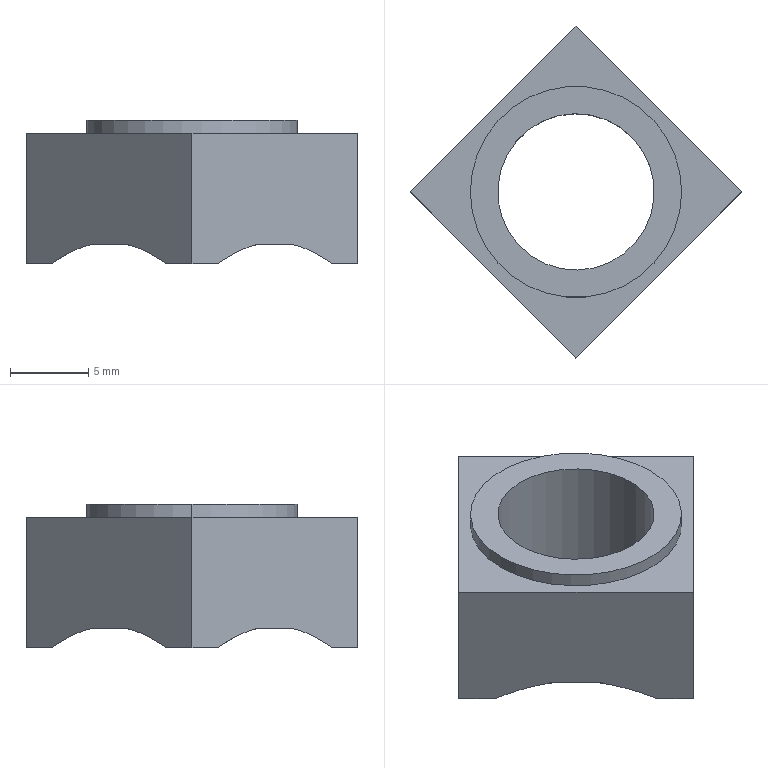Part | STEP file | Q37110 | 1 solid | 20 faces | box 21.213 x 21.213 x 9.167 mm | volume 1120 mm3 | plane 11 | cone 5 | cylinder 4 | commonest cylinder face diameters 10 x2 13.5 x2
STEP:
#1=CARTESIAN_POINT('',(4.237,6.369,0.));
#2=VERTEX_POINT('',#1);
#3=CARTESIAN_POINT('',(6.369,4.237,0.));
#4=VERTEX_POINT('',#3);
#5=CARTESIAN_POINT('',(5.303,5.303,0.));
#6=DIRECTION('',(0.7071,-0.7071,0.));
#7=VECTOR('',#6,1.);
#8=LINE('',#5,#7);
#9=EDGE_CURVE('',#2,#4,#8,.T.);
#10=ORIENTED_EDGE('',*,*,#9,.T.);
#11=CARTESIAN_POINT('',(6.714,3.668,0.));
#12=VERTEX_POINT('',#11);
#13=CARTESIAN_POINT('',(0.,0.,0.));
#14=DIRECTION('',(0.,0.,1.));
#15=AXIS2_PLACEMENT_3D('',#13,#14,$);
#16=CIRCLE('',#15,7.65);
#17=EDGE_CURVE('',#12,#4,#16,.T.);
#18=ORIENTED_EDGE('',*,*,#17,.F.);
#19=CARTESIAN_POINT('',(6.369,-4.237,0.));
#20=VERTEX_POINT('',#19);
#21=CARTESIAN_POINT('',(0.,0.,0.));
#22=DIRECTION('',(0.,0.,1.));
#23=AXIS2_PLACEMENT_3D('',#21,#22,$);
#24=CIRCLE('',#23,7.65);
#25=EDGE_CURVE('',#20,#12,#24,.T.);
#26=ORIENTED_EDGE('',*,*,#25,.F.);
#27=CARTESIAN_POINT('',(4.237,-6.369,0.));
#28=VERTEX_POINT('',#27);
#29=CARTESIAN_POINT('',(5.303,-5.303,0.));
#30=DIRECTION('',(-0.7071,-0.7071,0.));
#31=VECTOR('',#30,1.);
#32=LINE('',#29,#31);
#33=EDGE_CURVE('',#20,#28,#32,.T.);
#34=ORIENTED_EDGE('',*,*,#33,.T.);
#35=CARTESIAN_POINT('',(-4.237,-6.369,0.));
#36=VERTEX_POINT('',#35);
#37=CARTESIAN_POINT('',(0.,0.,0.));
#38=DIRECTION('',(0.,0.,1.));
#39=AXIS2_PLACEMENT_3D('',#37,#38,$);
#40=CIRCLE('',#39,7.65);
#41=EDGE_CURVE('',#36,#28,#40,.T.);
#42=ORIENTED_EDGE('',*,*,#41,.F.);
#43=CARTESIAN_POINT('',(-6.369,-4.237,0.));
#44=VERTEX_POINT('',#43);
#45=CARTESIAN_POINT('',(-5.303,-5.303,0.));
#46=DIRECTION('',(0.7071,-0.7071,0.));
#47=VECTOR('',#46,1.);
#48=LINE('',#45,#47);
#49=EDGE_CURVE('',#44,#36,#48,.T.);
#50=ORIENTED_EDGE('',*,*,#49,.F.);
#51=CARTESIAN_POINT('',(-6.714,-3.668,0.));
#52=VERTEX_POINT('',#51);
#53=CARTESIAN_POINT('',(0.,0.,0.));
#54=DIRECTION('',(0.,0.,1.));
#55=AXIS2_PLACEMENT_3D('',#53,#54,$);
#56=CIRCLE('',#55,7.65);
#57=EDGE_CURVE('',#52,#44,#56,.T.);
#58=ORIENTED_EDGE('',*,*,#57,.F.);
#59=CARTESIAN_POINT('',(-6.369,4.237,0.));
#60=VERTEX_POINT('',#59);
#61=CARTESIAN_POINT('',(0.,0.,0.));
#62=DIRECTION('',(0.,0.,1.));
#63=AXIS2_PLACEMENT_3D('',#61,#62,$);
#64=CIRCLE('',#63,7.65);
#65=EDGE_CURVE('',#60,#52,#64,.T.);
#66=ORIENTED_EDGE('',*,*,#65,.F.);
#67=CARTESIAN_POINT('',(-4.237,6.369,0.));
#68=VERTEX_POINT('',#67);
#69=CARTESIAN_POINT('',(-5.303,5.303,0.));
#70=DIRECTION('',(0.7071,0.7071,0.));
#71=VECTOR('',#70,1.);
#72=LINE('',#69,#71);
#73=EDGE_CURVE('',#60,#68,#72,.T.);
#74=ORIENTED_EDGE('',*,*,#73,.T.);
#75=CARTESIAN_POINT('',(0.,0.,0.));
#76=DIRECTION('',(0.,0.,1.));
#77=AXIS2_PLACEMENT_3D('',#75,#76,$);
#78=CIRCLE('',#77,7.65);
#79=EDGE_CURVE('',#2,#68,#78,.T.);
#80=ORIENTED_EDGE('',*,*,#79,.F.);
#81=EDGE_LOOP('',(#10,#18,#26,#34,#42,#50,#58,#66,#74,#80));
#82=FACE_OUTER_BOUND('',#81,.T.);
#83=CARTESIAN_POINT('',(-4.388,2.397,0.));
#84=VERTEX_POINT('',#83);
#85=CARTESIAN_POINT('',(4.388,-2.397,0.));
#86=VERTEX_POINT('',#85);
#87=CARTESIAN_POINT('',(0.,0.,0.));
#88=DIRECTION('',(0.,0.,1.));
#89=AXIS2_PLACEMENT_3D('',#87,#88,$);
#90=CIRCLE('',#89,5.);
#91=EDGE_CURVE('',#84,#86,#90,.T.);
#92=ORIENTED_EDGE('',*,*,#91,.T.);
#93=CARTESIAN_POINT('',(0.,0.,0.));
#94=DIRECTION('',(0.,0.,1.));
#95=AXIS2_PLACEMENT_3D('',#93,#94,$);
#96=CIRCLE('',#95,5.);
#97=EDGE_CURVE('',#86,#84,#96,.T.);
#98=ORIENTED_EDGE('',*,*,#97,.T.);
#99=EDGE_LOOP('',(#92,#98));
#100=FACE_BOUND('',#99,.T.);
#101=CARTESIAN_POINT('',(0.,0.,0.));
#102=DIRECTION('',(0.,0.,1.));
#103=DIRECTION('',(0.8333,0.,0.));
#104=AXIS2_PLACEMENT_3D('',#101,#102,#103);
#105=PLANE('',#104);
#106=ADVANCED_FACE('',(#82,#100),#105,.F.);
#107=CARTESIAN_POINT('',(-1.61,8.997,-1.25));
#108=VERTEX_POINT('',#107);
#109=CARTESIAN_POINT('',(-4.237,6.369,0.));
#110=CARTESIAN_POINT('',(-3.9,6.707,-0.07892));
#111=CARTESIAN_POINT('',(-3.552,7.054,-0.1902));
#112=CARTESIAN_POINT('',(-3.189,7.418,-0.337));
#113=CARTESIAN_POINT('',(-2.669,7.938,-0.5899));
#114=CARTESIAN_POINT('',(-2.088,8.519,-0.9383));
#115=CARTESIAN_POINT('',(-1.934,8.673,-1.035));
#116=CARTESIAN_POINT('',(-1.775,8.832,-1.138));
#117=CARTESIAN_POINT('',(-1.61,8.997,-1.25));
#118=B_SPLINE_CURVE_WITH_KNOTS('',5,(#109,#110,#111,#112,#113,#114,#115,#116,#117),.UNSPECIFIED.,.F.,.U.,(6,3,6),(0.,30.729,41.356),.UNSPECIFIED.);
#119=EDGE_CURVE('',#68,#108,#118,.T.);
#120=ORIENTED_EDGE('',*,*,#119,.F.);
#121=ORIENTED_EDGE('',*,*,#73,.F.);
#122=CARTESIAN_POINT('',(-8.997,1.61,-1.25));
#123=VERTEX_POINT('',#122);
#124=CARTESIAN_POINT('',(-6.369,4.237,0.));
#125=CARTESIAN_POINT('',(-6.707,3.9,-0.07892));
#126=CARTESIAN_POINT('',(-7.054,3.552,-0.1902));
#127=CARTESIAN_POINT('',(-7.418,3.189,-0.337));
#128=CARTESIAN_POINT('',(-7.938,2.669,-0.5899));
#129=CARTESIAN_POINT('',(-8.519,2.088,-0.9383));
#130=CARTESIAN_POINT('',(-8.673,1.934,-1.035));
#131=CARTESIAN_POINT('',(-8.832,1.775,-1.138));
#132=CARTESIAN_POINT('',(-8.997,1.61,-1.25));
#133=B_SPLINE_CURVE_WITH_KNOTS('',5,(#124,#125,#126,#127,#128,#129,#130,#131,#132),.UNSPECIFIED.,.F.,.U.,(6,3,6),(0.,30.729,41.356),.UNSPECIFIED.);
#134=EDGE_CURVE('',#60,#123,#133,.T.);
#135=ORIENTED_EDGE('',*,*,#134,.T.);
#136=CARTESIAN_POINT('',(-10.607,0.,-1.25));
#137=VERTEX_POINT('',#136);
#138=CARTESIAN_POINT('',(-9.802,0.8049,-1.25));
#139=DIRECTION('',(0.7071,0.7071,0.));
#140=VECTOR('',#139,1.);
#141=LINE('',#138,#140);
#142=EDGE_CURVE('',#123,#137,#141,.F.);
#143=ORIENTED_EDGE('',*,*,#142,.T.);
#144=CARTESIAN_POINT('',(-10.607,0.,7.083));
#145=VERTEX_POINT('',#144);
#146=CARTESIAN_POINT('',(-10.607,0.,2.917));
#147=DIRECTION('',(0.,0.,1.));
#148=VECTOR('',#147,1.);
#149=LINE('',#146,#148);
#150=EDGE_CURVE('',#137,#145,#149,.T.);
#151=ORIENTED_EDGE('',*,*,#150,.T.);
#152=CARTESIAN_POINT('',(0.,10.607,7.083));
#153=VERTEX_POINT('',#152);
#154=CARTESIAN_POINT('',(-5.303,5.303,7.083));
#155=DIRECTION('',(0.7071,0.7071,0.));
#156=VECTOR('',#155,1.);
#157=LINE('',#154,#156);
#158=EDGE_CURVE('',#153,#145,#157,.F.);
#159=ORIENTED_EDGE('',*,*,#158,.F.);
#160=CARTESIAN_POINT('',(0.,10.607,-1.25));
#161=VERTEX_POINT('',#160);
#162=CARTESIAN_POINT('',(0.,10.607,2.917));
#163=DIRECTION('',(0.,0.,1.));
#164=VECTOR('',#163,1.);
#165=LINE('',#162,#164);
#166=EDGE_CURVE('',#161,#153,#165,.T.);
#167=ORIENTED_EDGE('',*,*,#166,.F.);
#168=CARTESIAN_POINT('',(-0.8049,9.802,-1.25));
#169=DIRECTION('',(0.7071,0.7071,0.));
#170=VECTOR('',#169,1.);
#171=LINE('',#168,#170);
#172=EDGE_CURVE('',#161,#108,#171,.F.);
#173=ORIENTED_EDGE('',*,*,#172,.T.);
#174=EDGE_LOOP('',(#120,#121,#135,#143,#151,#159,#167,#173));
#175=FACE_OUTER_BOUND('',#174,.T.);
#176=CARTESIAN_POINT('',(-10.607,0.,0.));
#177=DIRECTION('',(0.7071,-0.7071,0.));
#178=DIRECTION('',(0.5893,0.5893,0.));
#179=AXIS2_PLACEMENT_3D('',#176,#177,#178);
#180=PLANE('',#179);
#181=ADVANCED_FACE('',(#175),#180,.F.);
#182=CARTESIAN_POINT('',(1.61,-8.997,-1.25));
#183=VERTEX_POINT('',#182);
#184=CARTESIAN_POINT('',(4.237,-6.369,0.));
#185=CARTESIAN_POINT('',(3.9,-6.707,-0.07892));
#186=CARTESIAN_POINT('',(3.552,-7.054,-0.1902));
#187=CARTESIAN_POINT('',(3.189,-7.418,-0.337));
#188=CARTESIAN_POINT('',(2.669,-7.938,-0.5899));
#189=CARTESIAN_POINT('',(2.088,-8.519,-0.9383));
#190=CARTESIAN_POINT('',(1.934,-8.673,-1.035));
#191=CARTESIAN_POINT('',(1.775,-8.832,-1.138));
#192=CARTESIAN_POINT('',(1.61,-8.997,-1.25));
#193=B_SPLINE_CURVE_WITH_KNOTS('',5,(#184,#185,#186,#187,#188,#189,#190,#191,#192),.UNSPECIFIED.,.F.,.U.,(6,3,6),(0.,30.729,41.356),.UNSPECIFIED.);
#194=EDGE_CURVE('',#28,#183,#193,.T.);
#195=ORIENTED_EDGE('',*,*,#194,.F.);
#196=ORIENTED_EDGE('',*,*,#33,.F.);
#197=CARTESIAN_POINT('',(8.997,-1.61,-1.25));
#198=VERTEX_POINT('',#197);
#199=CARTESIAN_POINT('',(6.369,-4.237,0.));
#200=CARTESIAN_POINT('',(6.707,-3.9,-0.07892));
#201=CARTESIAN_POINT('',(7.054,-3.552,-0.1902));
#202=CARTESIAN_POINT('',(7.418,-3.189,-0.337));
#203=CARTESIAN_POINT('',(7.938,-2.669,-0.5899));
#204=CARTESIAN_POINT('',(8.519,-2.088,-0.9383));
#205=CARTESIAN_POINT('',(8.673,-1.934,-1.035));
#206=CARTESIAN_POINT('',(8.832,-1.775,-1.138));
#207=CARTESIAN_POINT('',(8.997,-1.61,-1.25));
#208=B_SPLINE_CURVE_WITH_KNOTS('',5,(#199,#200,#201,#202,#203,#204,#205,#206,#207),.UNSPECIFIED.,.F.,.U.,(6,3,6),(0.,30.729,41.356),.UNSPECIFIED.);
#209=EDGE_CURVE('',#20,#198,#208,.T.);
#210=ORIENTED_EDGE('',*,*,#209,.T.);
#211=CARTESIAN_POINT('',(10.607,0.,-1.25));
#212=VERTEX_POINT('',#211);
#213=CARTESIAN_POINT('',(9.802,-0.8049,-1.25));
#214=DIRECTION('',(-0.7071,-0.7071,0.));
#215=VECTOR('',#214,1.);
#216=LINE('',#213,#215);
#217=EDGE_CURVE('',#198,#212,#216,.F.);
#218=ORIENTED_EDGE('',*,*,#217,.T.);
#219=CARTESIAN_POINT('',(10.607,0.,7.083));
#220=VERTEX_POINT('',#219);
#221=CARTESIAN_POINT('',(10.607,0.,2.917));
#222=DIRECTION('',(0.,0.,1.));
#223=VECTOR('',#222,1.);
#224=LINE('',#221,#223);
#225=EDGE_CURVE('',#212,#220,#224,.T.);
#226=ORIENTED_EDGE('',*,*,#225,.T.);
#227=CARTESIAN_POINT('',(0.,-10.607,7.083));
#228=VERTEX_POINT('',#227);
#229=CARTESIAN_POINT('',(5.303,-5.303,7.083));
#230=DIRECTION('',(-0.7071,-0.7071,0.));
#231=VECTOR('',#230,1.);
#232=LINE('',#229,#231);
#233=EDGE_CURVE('',#228,#220,#232,.F.);
#234=ORIENTED_EDGE('',*,*,#233,.F.);
#235=CARTESIAN_POINT('',(0.,-10.607,-1.25));
#236=VERTEX_POINT('',#235);
#237=CARTESIAN_POINT('',(0.,-10.607,2.917));
#238=DIRECTION('',(0.,0.,1.));
#239=VECTOR('',#238,1.);
#240=LINE('',#237,#239);
#241=EDGE_CURVE('',#236,#228,#240,.T.);
#242=ORIENTED_EDGE('',*,*,#241,.F.);
#243=CARTESIAN_POINT('',(0.8049,-9.802,-1.25));
#244=DIRECTION('',(-0.7071,-0.7071,0.));
#245=VECTOR('',#244,1.);
#246=LINE('',#243,#245);
#247=EDGE_CURVE('',#236,#183,#246,.F.);
#248=ORIENTED_EDGE('',*,*,#247,.T.);
#249=EDGE_LOOP('',(#195,#196,#210,#218,#226,#234,#242,#248));
#250=FACE_OUTER_BOUND('',#249,.T.);
#251=CARTESIAN_POINT('',(10.607,0.,0.));
#252=DIRECTION('',(-0.7071,0.7071,0.));
#253=DIRECTION('',(-0.5893,-0.5893,0.));
#254=AXIS2_PLACEMENT_3D('',#251,#252,#253);
#255=PLANE('',#254);
#256=ADVANCED_FACE('',(#250),#255,.F.);
#257=CARTESIAN_POINT('',(6.859,3.747,-0.1394));
#258=VERTEX_POINT('',#257);
#259=CARTESIAN_POINT('',(8.997,1.61,-1.25));
#260=VERTEX_POINT('',#259);
#261=CARTESIAN_POINT('',(6.859,3.747,-0.1394));
#262=CARTESIAN_POINT('',(7.213,3.394,-0.2575));
#263=CARTESIAN_POINT('',(7.581,3.025,-0.4115));
#264=CARTESIAN_POINT('',(7.972,2.634,-0.6064));
#265=CARTESIAN_POINT('',(8.418,2.188,-0.8643));
#266=CARTESIAN_POINT('',(8.915,1.691,-1.195));
#267=CARTESIAN_POINT('',(8.942,1.664,-1.213));
#268=CARTESIAN_POINT('',(8.969,1.637,-1.231));
#269=CARTESIAN_POINT('',(8.997,1.61,-1.25));
#270=B_SPLINE_CURVE_WITH_KNOTS('',5,(#261,#262,#263,#264,#265,#266,#267,#268,#269),.UNSPECIFIED.,.F.,.U.,(6,3,6),(0.,30.843,32.608),.UNSPECIFIED.);
#271=EDGE_CURVE('',#258,#260,#270,.T.);
#272=ORIENTED_EDGE('',*,*,#271,.F.);
#273=CARTESIAN_POINT('',(6.369,4.237,0.));
#274=CARTESIAN_POINT('',(6.465,4.141,-0.02247));
#275=CARTESIAN_POINT('',(6.562,4.044,-0.04757));
#276=CARTESIAN_POINT('',(6.66,3.946,-0.07536));
#277=CARTESIAN_POINT('',(6.759,3.847,-0.1059));
#278=CARTESIAN_POINT('',(6.859,3.747,-0.1394));
#279=B_SPLINE_CURVE_WITH_KNOTS('',5,(#273,#274,#275,#276,#277,#278),.UNSPECIFIED.,.F.,.U.,(6,6),(0.,8.749),.UNSPECIFIED.);
#280=EDGE_CURVE('',#4,#258,#279,.T.);
#281=ORIENTED_EDGE('',*,*,#280,.F.);
#282=ORIENTED_EDGE('',*,*,#9,.F.);
#283=CARTESIAN_POINT('',(1.61,8.997,-1.25));
#284=VERTEX_POINT('',#283);
#285=CARTESIAN_POINT('',(4.237,6.369,0.));
#286=CARTESIAN_POINT('',(3.9,6.707,-0.07892));
#287=CARTESIAN_POINT('',(3.552,7.054,-0.1902));
#288=CARTESIAN_POINT('',(3.189,7.418,-0.337));
#289=CARTESIAN_POINT('',(2.669,7.938,-0.5899));
#290=CARTESIAN_POINT('',(2.088,8.519,-0.9383));
#291=CARTESIAN_POINT('',(1.934,8.673,-1.035));
#292=CARTESIAN_POINT('',(1.775,8.832,-1.138));
#293=CARTESIAN_POINT('',(1.61,8.997,-1.25));
#294=B_SPLINE_CURVE_WITH_KNOTS('',5,(#285,#286,#287,#288,#289,#290,#291,#292,#293),.UNSPECIFIED.,.F.,.U.,(6,3,6),(0.,30.729,41.356),.UNSPECIFIED.);
#295=EDGE_CURVE('',#2,#284,#294,.T.);
#296=ORIENTED_EDGE('',*,*,#295,.T.);
#297=CARTESIAN_POINT('',(0.8049,9.802,-1.25));
#298=DIRECTION('',(0.7071,-0.7071,0.));
#299=VECTOR('',#298,1.);
#300=LINE('',#297,#299);
#301=EDGE_CURVE('',#284,#161,#300,.F.);
#302=ORIENTED_EDGE('',*,*,#301,.T.);
#303=ORIENTED_EDGE('',*,*,#166,.T.);
#304=CARTESIAN_POINT('',(5.303,5.303,7.083));
#305=DIRECTION('',(0.7071,-0.7071,0.));
#306=VECTOR('',#305,1.);
#307=LINE('',#304,#306);
#308=EDGE_CURVE('',#220,#153,#307,.F.);
#309=ORIENTED_EDGE('',*,*,#308,.F.);
#310=ORIENTED_EDGE('',*,*,#225,.F.);
#311=CARTESIAN_POINT('',(9.802,0.8049,-1.25));
#312=DIRECTION('',(0.7071,-0.7071,0.));
#313=VECTOR('',#312,1.);
#314=LINE('',#311,#313);
#315=EDGE_CURVE('',#212,#260,#314,.F.);
#316=ORIENTED_EDGE('',*,*,#315,.T.);
#317=EDGE_LOOP('',(#272,#281,#282,#296,#302,#303,#309,#310,#316));
#318=FACE_OUTER_BOUND('',#317,.T.);
#319=CARTESIAN_POINT('',(0.,10.607,0.));
#320=DIRECTION('',(-0.7071,-0.7071,0.));
#321=DIRECTION('',(0.5893,-0.5893,0.));
#322=AXIS2_PLACEMENT_3D('',#319,#320,#321);
#323=PLANE('',#322);
#324=ADVANCED_FACE('',(#318),#323,.F.);
#325=ORIENTED_EDGE('',*,*,#97,.F.);
#326=CARTESIAN_POINT('',(4.388,-2.397,7.917));
#327=VERTEX_POINT('',#326);
#328=CARTESIAN_POINT('',(4.388,-2.397,3.333));
#329=DIRECTION('',(0.,0.,-1.));
#330=VECTOR('',#329,1.);
#331=LINE('',#328,#330);
#332=EDGE_CURVE('',#86,#327,#331,.F.);
#333=ORIENTED_EDGE('',*,*,#332,.T.);
#334=CARTESIAN_POINT('',(-4.388,2.397,7.917));
#335=VERTEX_POINT('',#334);
#336=CARTESIAN_POINT('',(0.,0.,7.917));
#337=DIRECTION('',(0.,0.,-1.));
#338=AXIS2_PLACEMENT_3D('',#336,#337,$);
#339=CIRCLE('',#338,5.);
#340=EDGE_CURVE('',#327,#335,#339,.F.);
#341=ORIENTED_EDGE('',*,*,#340,.T.);
#342=CARTESIAN_POINT('',(-4.388,2.397,3.333));
#343=DIRECTION('',(0.,0.,-1.));
#344=VECTOR('',#343,1.);
#345=LINE('',#342,#344);
#346=EDGE_CURVE('',#84,#335,#345,.F.);
#347=ORIENTED_EDGE('',*,*,#346,.F.);
#348=EDGE_LOOP('',(#325,#333,#341,#347));
#349=FACE_OUTER_BOUND('',#348,.T.);
#350=CARTESIAN_POINT('',(0.,0.,7.667));
#351=DIRECTION('',(0.,0.,-1.));
#352=DIRECTION('',(0.8776,-0.4794,0.));
#353=AXIS2_PLACEMENT_3D('',#350,#351,#352);
#354=CYLINDRICAL_SURFACE('',#353,5.);
#355=ADVANCED_FACE('',(#349),#354,.F.);
#356=ORIENTED_EDGE('',*,*,#91,.F.);
#357=ORIENTED_EDGE('',*,*,#346,.T.);
#358=CARTESIAN_POINT('',(0.,0.,7.917));
#359=DIRECTION('',(0.,0.,-1.));
#360=AXIS2_PLACEMENT_3D('',#358,#359,$);
#361=CIRCLE('',#360,5.);
#362=EDGE_CURVE('',#335,#327,#361,.F.);
#363=ORIENTED_EDGE('',*,*,#362,.T.);
#364=ORIENTED_EDGE('',*,*,#332,.F.);
#365=EDGE_LOOP('',(#356,#357,#363,#364));
#366=FACE_OUTER_BOUND('',#365,.T.);
#367=ADVANCED_FACE('',(#366),#354,.F.);
#368=CARTESIAN_POINT('',(0.,0.,-1.25));
#369=DIRECTION('',(0.,0.,1.));
#370=AXIS2_PLACEMENT_3D('',#368,#369,$);
#371=CIRCLE('',#370,9.14);
#372=EDGE_CURVE('',#284,#108,#371,.T.);
#373=ORIENTED_EDGE('',*,*,#372,.T.);
#374=ORIENTED_EDGE('',*,*,#172,.F.);
#375=ORIENTED_EDGE('',*,*,#301,.F.);
#376=EDGE_LOOP('',(#373,#374,#375));
#377=FACE_OUTER_BOUND('',#376,.T.);
#378=CARTESIAN_POINT('',(0.,0.,-1.25));
#379=DIRECTION('',(0.,0.,1.));
#380=DIRECTION('',(0.8333,0.,0.));
#381=AXIS2_PLACEMENT_3D('',#378,#379,#380);
#382=PLANE('',#381);
#383=ADVANCED_FACE('',(#377),#382,.F.);
#384=CARTESIAN_POINT('',(-8.997,-1.61,-1.25));
#385=VERTEX_POINT('',#384);
#386=CARTESIAN_POINT('',(0.,0.,-1.25));
#387=DIRECTION('',(0.,0.,1.));
#388=AXIS2_PLACEMENT_3D('',#386,#387,$);
#389=CIRCLE('',#388,9.14);
#390=EDGE_CURVE('',#123,#385,#389,.T.);
#391=ORIENTED_EDGE('',*,*,#390,.T.);
#392=CARTESIAN_POINT('',(-9.802,-0.8049,-1.25));
#393=DIRECTION('',(-0.7071,0.7071,0.));
#394=VECTOR('',#393,1.);
#395=LINE('',#392,#394);
#396=EDGE_CURVE('',#137,#385,#395,.F.);
#397=ORIENTED_EDGE('',*,*,#396,.F.);
#398=ORIENTED_EDGE('',*,*,#142,.F.);
#399=EDGE_LOOP('',(#391,#397,#398));
#400=FACE_OUTER_BOUND('',#399,.T.);
#401=ADVANCED_FACE('',(#400),#382,.F.);
#402=CARTESIAN_POINT('',(-1.61,-8.997,-1.25));
#403=VERTEX_POINT('',#402);
#404=CARTESIAN_POINT('',(0.,0.,-1.25));
#405=DIRECTION('',(0.,0.,1.));
#406=AXIS2_PLACEMENT_3D('',#404,#405,$);
#407=CIRCLE('',#406,9.14);
#408=EDGE_CURVE('',#403,#183,#407,.T.);
#409=ORIENTED_EDGE('',*,*,#408,.T.);
#410=ORIENTED_EDGE('',*,*,#247,.F.);
#411=CARTESIAN_POINT('',(-0.8049,-9.802,-1.25));
#412=DIRECTION('',(-0.7071,0.7071,0.));
#413=VECTOR('',#412,1.);
#414=LINE('',#411,#413);
#415=EDGE_CURVE('',#403,#236,#414,.F.);
#416=ORIENTED_EDGE('',*,*,#415,.F.);
#417=EDGE_LOOP('',(#409,#410,#416));
#418=FACE_OUTER_BOUND('',#417,.T.);
#419=ADVANCED_FACE('',(#418),#382,.F.);
#420=CARTESIAN_POINT('',(0.,0.,-1.25));
#421=DIRECTION('',(0.,0.,1.));
#422=AXIS2_PLACEMENT_3D('',#420,#421,$);
#423=CIRCLE('',#422,9.14);
#424=EDGE_CURVE('',#198,#260,#423,.T.);
#425=ORIENTED_EDGE('',*,*,#424,.T.);
#426=ORIENTED_EDGE('',*,*,#315,.F.);
#427=ORIENTED_EDGE('',*,*,#217,.F.);
#428=EDGE_LOOP('',(#425,#426,#427));
#429=FACE_OUTER_BOUND('',#428,.T.);
#430=ADVANCED_FACE('',(#429),#382,.F.);
#431=CARTESIAN_POINT('',(6.75,0.,7.917));
#432=VERTEX_POINT('',#431);
#433=CARTESIAN_POINT('',(-6.75,0.,7.917));
#434=VERTEX_POINT('',#433);
#435=CARTESIAN_POINT('',(0.,0.,7.917));
#436=DIRECTION('',(0.,0.,1.));
#437=AXIS2_PLACEMENT_3D('',#435,#436,$);
#438=CIRCLE('',#437,6.75);
#439=EDGE_CURVE('',#432,#434,#438,.T.);
#440=ORIENTED_EDGE('',*,*,#439,.T.);
#441=CARTESIAN_POINT('',(0.,0.,7.917));
#442=DIRECTION('',(0.,0.,1.));
#443=AXIS2_PLACEMENT_3D('',#441,#442,$);
#444=CIRCLE('',#443,6.75);
#445=EDGE_CURVE('',#434,#432,#444,.T.);
#446=ORIENTED_EDGE('',*,*,#445,.T.);
#447=EDGE_LOOP('',(#440,#446));
#448=FACE_OUTER_BOUND('',#447,.T.);
#449=ORIENTED_EDGE('',*,*,#362,.F.);
#450=ORIENTED_EDGE('',*,*,#340,.F.);
#451=EDGE_LOOP('',(#449,#450));
#452=FACE_BOUND('',#451,.T.);
#453=CARTESIAN_POINT('',(0.,0.,7.917));
#454=DIRECTION('',(0.,0.,1.));
#455=DIRECTION('',(0.8333,0.,0.));
#456=AXIS2_PLACEMENT_3D('',#453,#454,#455);
#457=PLANE('',#456);
#458=ADVANCED_FACE('',(#448,#452),#457,.T.);
#459=CARTESIAN_POINT('',(6.75,0.,7.083));
#460=VERTEX_POINT('',#459);
#461=CARTESIAN_POINT('',(6.75,0.,7.5));
#462=DIRECTION('',(0.,0.,1.));
#463=VECTOR('',#462,1.);
#464=LINE('',#461,#463);
#465=EDGE_CURVE('',#460,#432,#464,.T.);
#466=ORIENTED_EDGE('',*,*,#465,.F.);
#467=CARTESIAN_POINT('',(-6.75,0.,7.083));
#468=VERTEX_POINT('',#467);
#469=CARTESIAN_POINT('',(0.,0.,7.083));
#470=DIRECTION('',(0.,0.,1.));
#471=AXIS2_PLACEMENT_3D('',#469,#470,$);
#472=CIRCLE('',#471,6.75);
#473=EDGE_CURVE('',#460,#468,#472,.T.);
#474=ORIENTED_EDGE('',*,*,#473,.T.);
#475=CARTESIAN_POINT('',(-6.75,0.,7.5));
#476=DIRECTION('',(0.,0.,1.));
#477=VECTOR('',#476,1.);
#478=LINE('',#475,#477);
#479=EDGE_CURVE('',#468,#434,#478,.T.);
#480=ORIENTED_EDGE('',*,*,#479,.T.);
#481=ORIENTED_EDGE('',*,*,#439,.F.);
#482=EDGE_LOOP('',(#466,#474,#480,#481));
#483=FACE_OUTER_BOUND('',#482,.T.);
#484=CARTESIAN_POINT('',(0.,0.,7.5));
#485=DIRECTION('',(0.,0.,1.));
#486=DIRECTION('',(1.,0.,0.));
#487=AXIS2_PLACEMENT_3D('',#484,#485,#486);
#488=CYLINDRICAL_SURFACE('',#487,6.75);
#489=ADVANCED_FACE('',(#483),#488,.T.);
#490=ORIENTED_EDGE('',*,*,#479,.F.);
#491=CARTESIAN_POINT('',(0.,0.,7.083));
#492=DIRECTION('',(0.,0.,1.));
#493=AXIS2_PLACEMENT_3D('',#491,#492,$);
#494=CIRCLE('',#493,6.75);
#495=EDGE_CURVE('',#468,#460,#494,.T.);
#496=ORIENTED_EDGE('',*,*,#495,.T.);
#497=ORIENTED_EDGE('',*,*,#465,.T.);
#498=ORIENTED_EDGE('',*,*,#445,.F.);
#499=EDGE_LOOP('',(#490,#496,#497,#498));
#500=FACE_OUTER_BOUND('',#499,.T.);
#501=ADVANCED_FACE('',(#500),#488,.T.);
#502=CARTESIAN_POINT('',(-5.303,-5.303,7.083));
#503=DIRECTION('',(-0.7071,0.7071,0.));
#504=VECTOR('',#503,1.);
#505=LINE('',#502,#504);
#506=EDGE_CURVE('',#145,#228,#505,.F.);
#507=ORIENTED_EDGE('',*,*,#506,.T.);
#508=ORIENTED_EDGE('',*,*,#233,.T.);
#509=ORIENTED_EDGE('',*,*,#308,.T.);
#510=ORIENTED_EDGE('',*,*,#158,.T.);
#511=EDGE_LOOP('',(#507,#508,#509,#510));
#512=FACE_OUTER_BOUND('',#511,.T.);
#513=ORIENTED_EDGE('',*,*,#473,.F.);
#514=ORIENTED_EDGE('',*,*,#495,.F.);
#515=EDGE_LOOP('',(#513,#514));
#516=FACE_BOUND('',#515,.T.);
#517=CARTESIAN_POINT('',(0.,0.,7.083));
#518=DIRECTION('',(0.,0.,1.));
#519=DIRECTION('',(0.8333,0.,0.));
#520=AXIS2_PLACEMENT_3D('',#517,#518,#519);
#521=PLANE('',#520);
#522=ADVANCED_FACE('',(#512,#516),#521,.T.);
#523=ORIENTED_EDGE('',*,*,#280,.T.);
#524=CARTESIAN_POINT('',(7.423,4.055,-0.6786));
#525=DIRECTION('',(0.6723,0.3673,-0.6428));
#526=VECTOR('',#525,1.);
#527=LINE('',#524,#526);
#528=EDGE_CURVE('',#12,#258,#527,.T.);
#529=ORIENTED_EDGE('',*,*,#528,.F.);
#530=ORIENTED_EDGE('',*,*,#17,.T.);
#531=EDGE_LOOP('',(#523,#529,#530));
#532=FACE_OUTER_BOUND('',#531,.T.);
#533=CARTESIAN_POINT('',(0.,0.,0.));
#534=DIRECTION('',(0.,0.,-1.));
#535=DIRECTION('',(0.8776,0.4794,0.));
#536=AXIS2_PLACEMENT_3D('',#533,#534,#535);
#537=CONICAL_SURFACE('',#536,7.65,0.8727);
#538=ADVANCED_FACE('',(#532),#537,.F.);
#539=ORIENTED_EDGE('',*,*,#271,.T.);
#540=ORIENTED_EDGE('',*,*,#424,.F.);
#541=ORIENTED_EDGE('',*,*,#209,.F.);
#542=ORIENTED_EDGE('',*,*,#25,.T.);
#543=ORIENTED_EDGE('',*,*,#528,.T.);
#544=EDGE_LOOP('',(#539,#540,#541,#542,#543));
#545=FACE_OUTER_BOUND('',#544,.T.);
#546=ADVANCED_FACE('',(#545),#537,.F.);
#547=ORIENTED_EDGE('',*,*,#194,.T.);
#548=ORIENTED_EDGE('',*,*,#408,.F.);
#549=CARTESIAN_POINT('',(-4.237,-6.369,0.));
#550=CARTESIAN_POINT('',(-3.67,-6.937,-0.1328));
#551=CARTESIAN_POINT('',(-3.07,-7.536,-0.3647));
#552=CARTESIAN_POINT('',(-2.411,-8.195,-0.7064));
#553=CARTESIAN_POINT('',(-1.61,-8.997,-1.25));
#554=B_SPLINE_CURVE_WITH_KNOTS('',4,(#549,#550,#551,#552,#553),.UNSPECIFIED.,.F.,.U.,(5,5),(0.,41.356),.UNSPECIFIED.);
#555=EDGE_CURVE('',#36,#403,#554,.T.);
#556=ORIENTED_EDGE('',*,*,#555,.F.);
#557=ORIENTED_EDGE('',*,*,#41,.T.);
#558=EDGE_LOOP('',(#547,#548,#556,#557));
#559=FACE_OUTER_BOUND('',#558,.T.);
#560=ADVANCED_FACE('',(#559),#537,.F.);
#561=CARTESIAN_POINT('',(-6.859,-3.747,-0.1394));
#562=VERTEX_POINT('',#561);
#563=CARTESIAN_POINT('',(-6.859,-3.747,-0.1394));
#564=CARTESIAN_POINT('',(-7.213,-3.394,-0.2575));
#565=CARTESIAN_POINT('',(-7.581,-3.025,-0.4115));
#566=CARTESIAN_POINT('',(-7.972,-2.634,-0.6064));
#567=CARTESIAN_POINT('',(-8.418,-2.188,-0.8643));
#568=CARTESIAN_POINT('',(-8.915,-1.691,-1.195));
#569=CARTESIAN_POINT('',(-8.942,-1.664,-1.213));
#570=CARTESIAN_POINT('',(-8.969,-1.637,-1.231));
#571=CARTESIAN_POINT('',(-8.997,-1.61,-1.25));
#572=B_SPLINE_CURVE_WITH_KNOTS('',5,(#563,#564,#565,#566,#567,#568,#569,#570,#571),.UNSPECIFIED.,.F.,.U.,(6,3,6),(0.,30.843,32.608),.UNSPECIFIED.);
#573=EDGE_CURVE('',#562,#385,#572,.T.);
#574=ORIENTED_EDGE('',*,*,#573,.F.);
#575=CARTESIAN_POINT('',(-6.369,-4.237,0.));
#576=CARTESIAN_POINT('',(-6.465,-4.141,-0.02247));
#577=CARTESIAN_POINT('',(-6.562,-4.044,-0.04757));
#578=CARTESIAN_POINT('',(-6.66,-3.946,-0.07536));
#579=CARTESIAN_POINT('',(-6.759,-3.847,-0.1059));
#580=CARTESIAN_POINT('',(-6.859,-3.747,-0.1394));
#581=B_SPLINE_CURVE_WITH_KNOTS('',5,(#575,#576,#577,#578,#579,#580),.UNSPECIFIED.,.F.,.U.,(6,6),(0.,8.749),.UNSPECIFIED.);
#582=EDGE_CURVE('',#44,#562,#581,.T.);
#583=ORIENTED_EDGE('',*,*,#582,.F.);
#584=ORIENTED_EDGE('',*,*,#49,.T.);
#585=ORIENTED_EDGE('',*,*,#555,.T.);
#586=ORIENTED_EDGE('',*,*,#415,.T.);
#587=ORIENTED_EDGE('',*,*,#241,.T.);
#588=ORIENTED_EDGE('',*,*,#506,.F.);
#589=ORIENTED_EDGE('',*,*,#150,.F.);
#590=ORIENTED_EDGE('',*,*,#396,.T.);
#591=EDGE_LOOP('',(#574,#583,#584,#585,#586,#587,#588,#589,#590));
#592=FACE_OUTER_BOUND('',#591,.T.);
#593=CARTESIAN_POINT('',(0.,-10.607,0.));
#594=DIRECTION('',(0.7071,0.7071,0.));
#595=DIRECTION('',(-0.5893,0.5893,0.));
#596=AXIS2_PLACEMENT_3D('',#593,#594,#595);
#597=PLANE('',#596);
#598=ADVANCED_FACE('',(#592),#597,.F.);
#599=ORIENTED_EDGE('',*,*,#119,.T.);
#600=ORIENTED_EDGE('',*,*,#372,.F.);
#601=ORIENTED_EDGE('',*,*,#295,.F.);
#602=ORIENTED_EDGE('',*,*,#79,.T.);
#603=EDGE_LOOP('',(#599,#600,#601,#602));
#604=FACE_OUTER_BOUND('',#603,.T.);
#605=ADVANCED_FACE('',(#604),#537,.F.);
#606=ORIENTED_EDGE('',*,*,#582,.T.);
#607=ORIENTED_EDGE('',*,*,#573,.T.);
#608=ORIENTED_EDGE('',*,*,#390,.F.);
#609=ORIENTED_EDGE('',*,*,#134,.F.);
#610=ORIENTED_EDGE('',*,*,#65,.T.);
#611=ORIENTED_EDGE('',*,*,#57,.T.);
#612=EDGE_LOOP('',(#606,#607,#608,#609,#610,#611));
#613=FACE_OUTER_BOUND('',#612,.T.);
#614=ADVANCED_FACE('',(#613),#537,.F.);
#615=CLOSED_SHELL('',(#106,#181,#256,#324,#355,#367,#383,#401,#419,#430,#458,#489,#501,#522,#538,#546,#560,#598,#605,#614));
#616=MANIFOLD_SOLID_BREP('',#615);
#617=(LENGTH_UNIT()NAMED_UNIT(*)SI_UNIT(.MILLI.,.METRE.));
#618=UNCERTAINTY_MEASURE_WITH_UNIT(LENGTH_MEASURE(0.005),#617,'','');
#619=(NAMED_UNIT(*)PLANE_ANGLE_UNIT()SI_UNIT($,.RADIAN.));
#620=(NAMED_UNIT(*)SI_UNIT($,.STERADIAN.)SOLID_ANGLE_UNIT());
#621=(GEOMETRIC_REPRESENTATION_CONTEXT(3)GLOBAL_UNCERTAINTY_ASSIGNED_CONTEXT((#618))GLOBAL_UNIT_ASSIGNED_CONTEXT((#617,#619,#620))REPRESENTATION_CONTEXT('',''));
#622=ADVANCED_BREP_SHAPE_REPRESENTATION('',(#616),#621);